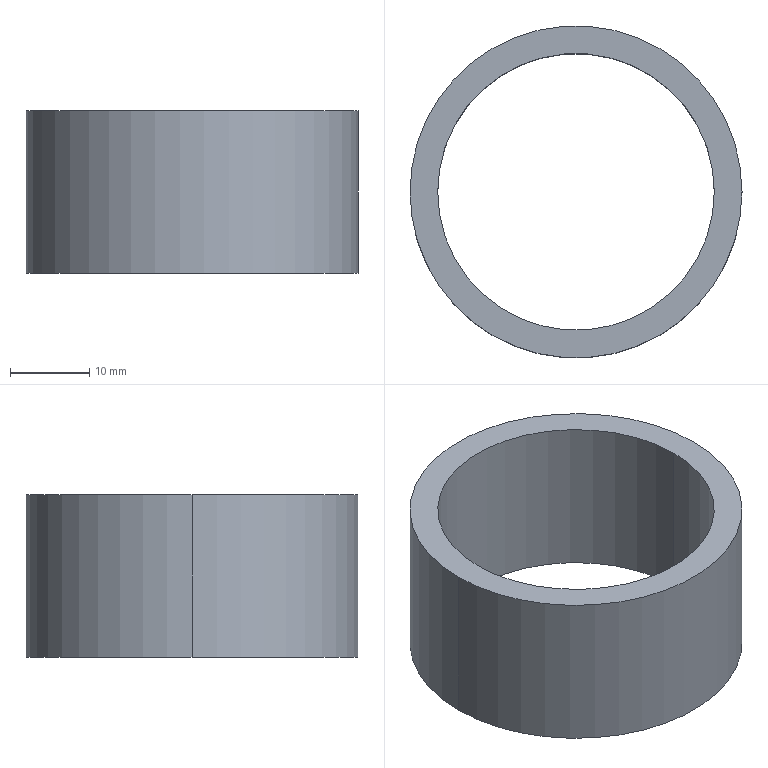Part | STEP file | 01-Spacer 51 | 1 solid | 6 faces | box 42 x 42 x 20.6 mm | volume 8721 mm3 | cylinder 4 | plane 2 | commonest cylinder face diameters 35 x2 42 x2
STEP:
#1=CARTESIAN_POINT('',(0.,0.,0.));
#2=DIRECTION('',(0.,0.,1.));
#3=DIRECTION('',(1.,0.,0.));
#4=AXIS2_PLACEMENT_3D('',#1,#2,#3);
#5=CARTESIAN_POINT('',(-17.5,0.,20.6));
#6=VERTEX_POINT('',#5);
#7=CARTESIAN_POINT('',(-17.5,0.,0.));
#8=VERTEX_POINT('',#7);
#9=CARTESIAN_POINT('',(-17.5,0.,20.6));
#10=DIRECTION('',(0.,0.,-1.));
#11=VECTOR('',#10,1.);
#12=LINE('',#9,#11);
#13=CARTESIAN_POINT('',(0.,0.,20.6));
#14=DIRECTION('',(0.,0.,-1.));
#15=DIRECTION('',(-1.,0.,0.));
#16=AXIS2_PLACEMENT_3D('',#13,#14,#15);
#17=CYLINDRICAL_SURFACE('',#16,17.5);
#18=CARTESIAN_POINT('',(6.283,0.));
#19=DIRECTION('',(0.,1.));
#20=VECTOR('',#19,1.);
#21=LINE('',#18,#20);
#22=(GEOMETRIC_REPRESENTATION_CONTEXT(2)PARAMETRIC_REPRESENTATION_CONTEXT()REPRESENTATION_CONTEXT('',''));
#23=DEFINITIONAL_REPRESENTATION('',(#21),#22);
#24=PCURVE('',#17,#23);
#25=CARTESIAN_POINT('',(0.,0.,20.6));
#26=DIRECTION('',(0.,0.,-1.));
#27=DIRECTION('',(-1.,0.,0.));
#28=AXIS2_PLACEMENT_3D('',#25,#26,#27);
#29=CYLINDRICAL_SURFACE('',#28,17.5);
#30=CARTESIAN_POINT('',(0.,0.));
#31=DIRECTION('',(0.,1.));
#32=VECTOR('',#31,1.);
#33=LINE('',#30,#32);
#34=(GEOMETRIC_REPRESENTATION_CONTEXT(2)PARAMETRIC_REPRESENTATION_CONTEXT()REPRESENTATION_CONTEXT('',''));
#35=DEFINITIONAL_REPRESENTATION('',(#33),#34);
#36=PCURVE('',#29,#35);
#37=SURFACE_CURVE('',#12,(#24,#36),.PCURVE_S1.);
#38=EDGE_CURVE('',#6,#8,#37,.T.);
#39=ORIENTED_EDGE('',*,*,#38,.T.);
#40=CARTESIAN_POINT('',(17.5,0.,0.));
#41=VERTEX_POINT('',#40);
#42=CARTESIAN_POINT('',(0.,0.,0.));
#43=DIRECTION('',(0.,0.,1.));
#44=DIRECTION('',(1.,0.,0.));
#45=AXIS2_PLACEMENT_3D('',#42,#43,#44);
#46=CIRCLE('',#45,17.5);
#47=CARTESIAN_POINT('',(9.425,20.6));
#48=DIRECTION('',(-1.,0.));
#49=VECTOR('',#48,1.);
#50=LINE('',#47,#49);
#51=(GEOMETRIC_REPRESENTATION_CONTEXT(2)PARAMETRIC_REPRESENTATION_CONTEXT()REPRESENTATION_CONTEXT('',''));
#52=DEFINITIONAL_REPRESENTATION('',(#50),#51);
#53=PCURVE('',#17,#52);
#54=CARTESIAN_POINT('',(0.,0.,0.));
#55=DIRECTION('',(0.,0.,1.));
#56=DIRECTION('',(1.,0.,0.));
#57=AXIS2_PLACEMENT_3D('',#54,#55,#56);
#58=PLANE('',#57);
#59=CARTESIAN_POINT('',(0.,0.));
#60=DIRECTION('',(1.,0.));
#61=AXIS2_PLACEMENT_2D('',#59,#60);
#62=CIRCLE('',#61,17.5);
#63=(GEOMETRIC_REPRESENTATION_CONTEXT(2)PARAMETRIC_REPRESENTATION_CONTEXT()REPRESENTATION_CONTEXT('',''));
#64=DEFINITIONAL_REPRESENTATION('',(#62),#63);
#65=PCURVE('',#58,#64);
#66=SURFACE_CURVE('',#46,(#53,#65),.PCURVE_S1.);
#67=EDGE_CURVE('',#8,#41,#66,.T.);
#68=ORIENTED_EDGE('',*,*,#67,.T.);
#69=CARTESIAN_POINT('',(17.5,0.,20.6));
#70=VERTEX_POINT('',#69);
#71=CARTESIAN_POINT('',(17.5,0.,20.6));
#72=DIRECTION('',(0.,0.,-1.));
#73=VECTOR('',#72,1.);
#74=LINE('',#71,#73);
#75=CARTESIAN_POINT('',(3.142,0.));
#76=DIRECTION('',(0.,1.));
#77=VECTOR('',#76,1.);
#78=LINE('',#75,#77);
#79=(GEOMETRIC_REPRESENTATION_CONTEXT(2)PARAMETRIC_REPRESENTATION_CONTEXT()REPRESENTATION_CONTEXT('',''));
#80=DEFINITIONAL_REPRESENTATION('',(#78),#79);
#81=PCURVE('',#17,#80);
#82=CARTESIAN_POINT('',(3.142,0.));
#83=DIRECTION('',(0.,1.));
#84=VECTOR('',#83,1.);
#85=LINE('',#82,#84);
#86=(GEOMETRIC_REPRESENTATION_CONTEXT(2)PARAMETRIC_REPRESENTATION_CONTEXT()REPRESENTATION_CONTEXT('',''));
#87=DEFINITIONAL_REPRESENTATION('',(#85),#86);
#88=PCURVE('',#29,#87);
#89=SURFACE_CURVE('',#74,(#81,#88),.PCURVE_S1.);
#90=EDGE_CURVE('',#70,#41,#89,.T.);
#91=ORIENTED_EDGE('',*,*,#90,.F.);
#92=CARTESIAN_POINT('',(0.,0.,20.6));
#93=DIRECTION('',(0.,0.,1.));
#94=DIRECTION('',(1.,0.,0.));
#95=AXIS2_PLACEMENT_3D('',#92,#93,#94);
#96=CIRCLE('',#95,17.5);
#97=CARTESIAN_POINT('',(9.425,0.));
#98=DIRECTION('',(-1.,0.));
#99=VECTOR('',#98,1.);
#100=LINE('',#97,#99);
#101=(GEOMETRIC_REPRESENTATION_CONTEXT(2)PARAMETRIC_REPRESENTATION_CONTEXT()REPRESENTATION_CONTEXT('',''));
#102=DEFINITIONAL_REPRESENTATION('',(#100),#101);
#103=PCURVE('',#17,#102);
#104=CARTESIAN_POINT('',(0.,0.,20.6));
#105=DIRECTION('',(0.,0.,1.));
#106=DIRECTION('',(1.,0.,0.));
#107=AXIS2_PLACEMENT_3D('',#104,#105,#106);
#108=PLANE('',#107);
#109=CARTESIAN_POINT('',(0.,0.));
#110=DIRECTION('',(1.,0.));
#111=AXIS2_PLACEMENT_2D('',#109,#110);
#112=CIRCLE('',#111,17.5);
#113=(GEOMETRIC_REPRESENTATION_CONTEXT(2)PARAMETRIC_REPRESENTATION_CONTEXT()REPRESENTATION_CONTEXT('',''));
#114=DEFINITIONAL_REPRESENTATION('',(#112),#113);
#115=PCURVE('',#108,#114);
#116=SURFACE_CURVE('',#96,(#103,#115),.PCURVE_S1.);
#117=EDGE_CURVE('',#6,#70,#116,.T.);
#118=ORIENTED_EDGE('',*,*,#117,.F.);
#119=EDGE_LOOP('',(#39,#68,#91,#118));
#120=FACE_BOUND('',#119,.F.);
#121=ADVANCED_FACE('',(#120),#17,.F.);
#122=CARTESIAN_POINT('',(21.,0.,20.6));
#123=VERTEX_POINT('',#122);
#124=CARTESIAN_POINT('',(-21.,0.,20.6));
#125=VERTEX_POINT('',#124);
#126=CARTESIAN_POINT('',(0.,0.,20.6));
#127=DIRECTION('',(0.,0.,1.));
#128=DIRECTION('',(1.,0.,0.));
#129=AXIS2_PLACEMENT_3D('',#126,#127,#128);
#130=CIRCLE('',#129,21.);
#131=CARTESIAN_POINT('',(0.,0.,20.6));
#132=DIRECTION('',(0.,0.,-1.));
#133=DIRECTION('',(-1.,0.,0.));
#134=AXIS2_PLACEMENT_3D('',#131,#132,#133);
#135=CYLINDRICAL_SURFACE('',#134,21.);
#136=CARTESIAN_POINT('',(3.142,0.));
#137=DIRECTION('',(-1.,0.));
#138=VECTOR('',#137,1.);
#139=LINE('',#136,#138);
#140=(GEOMETRIC_REPRESENTATION_CONTEXT(2)PARAMETRIC_REPRESENTATION_CONTEXT()REPRESENTATION_CONTEXT('',''));
#141=DEFINITIONAL_REPRESENTATION('',(#139),#140);
#142=PCURVE('',#135,#141);
#143=CARTESIAN_POINT('',(0.,0.));
#144=DIRECTION('',(1.,0.));
#145=AXIS2_PLACEMENT_2D('',#143,#144);
#146=CIRCLE('',#145,21.);
#147=(GEOMETRIC_REPRESENTATION_CONTEXT(2)PARAMETRIC_REPRESENTATION_CONTEXT()REPRESENTATION_CONTEXT('',''));
#148=DEFINITIONAL_REPRESENTATION('',(#146),#147);
#149=PCURVE('',#108,#148);
#150=SURFACE_CURVE('',#130,(#142,#149),.PCURVE_S1.);
#151=EDGE_CURVE('',#123,#125,#150,.T.);
#152=ORIENTED_EDGE('',*,*,#151,.F.);
#153=CARTESIAN_POINT('',(21.,0.,0.));
#154=VERTEX_POINT('',#153);
#155=CARTESIAN_POINT('',(21.,0.,20.6));
#156=DIRECTION('',(0.,0.,-1.));
#157=VECTOR('',#156,1.);
#158=LINE('',#155,#157);
#159=CARTESIAN_POINT('',(3.142,0.));
#160=DIRECTION('',(0.,1.));
#161=VECTOR('',#160,1.);
#162=LINE('',#159,#161);
#163=(GEOMETRIC_REPRESENTATION_CONTEXT(2)PARAMETRIC_REPRESENTATION_CONTEXT()REPRESENTATION_CONTEXT('',''));
#164=DEFINITIONAL_REPRESENTATION('',(#162),#163);
#165=PCURVE('',#135,#164);
#166=CARTESIAN_POINT('',(0.,0.,20.6));
#167=DIRECTION('',(0.,0.,-1.));
#168=DIRECTION('',(-1.,0.,0.));
#169=AXIS2_PLACEMENT_3D('',#166,#167,#168);
#170=CYLINDRICAL_SURFACE('',#169,21.);
#171=CARTESIAN_POINT('',(3.142,0.));
#172=DIRECTION('',(0.,1.));
#173=VECTOR('',#172,1.);
#174=LINE('',#171,#173);
#175=(GEOMETRIC_REPRESENTATION_CONTEXT(2)PARAMETRIC_REPRESENTATION_CONTEXT()REPRESENTATION_CONTEXT('',''));
#176=DEFINITIONAL_REPRESENTATION('',(#174),#175);
#177=PCURVE('',#170,#176);
#178=SURFACE_CURVE('',#158,(#165,#177),.PCURVE_S1.);
#179=EDGE_CURVE('',#123,#154,#178,.T.);
#180=ORIENTED_EDGE('',*,*,#179,.T.);
#181=CARTESIAN_POINT('',(-21.,0.,0.));
#182=VERTEX_POINT('',#181);
#183=CARTESIAN_POINT('',(0.,0.,0.));
#184=DIRECTION('',(0.,0.,1.));
#185=DIRECTION('',(1.,0.,0.));
#186=AXIS2_PLACEMENT_3D('',#183,#184,#185);
#187=CIRCLE('',#186,21.);
#188=CARTESIAN_POINT('',(3.142,20.6));
#189=DIRECTION('',(-1.,0.));
#190=VECTOR('',#189,1.);
#191=LINE('',#188,#190);
#192=(GEOMETRIC_REPRESENTATION_CONTEXT(2)PARAMETRIC_REPRESENTATION_CONTEXT()REPRESENTATION_CONTEXT('',''));
#193=DEFINITIONAL_REPRESENTATION('',(#191),#192);
#194=PCURVE('',#135,#193);
#195=CARTESIAN_POINT('',(0.,0.));
#196=DIRECTION('',(1.,0.));
#197=AXIS2_PLACEMENT_2D('',#195,#196);
#198=CIRCLE('',#197,21.);
#199=(GEOMETRIC_REPRESENTATION_CONTEXT(2)PARAMETRIC_REPRESENTATION_CONTEXT()REPRESENTATION_CONTEXT('',''));
#200=DEFINITIONAL_REPRESENTATION('',(#198),#199);
#201=PCURVE('',#58,#200);
#202=SURFACE_CURVE('',#187,(#194,#201),.PCURVE_S1.);
#203=EDGE_CURVE('',#154,#182,#202,.T.);
#204=ORIENTED_EDGE('',*,*,#203,.T.);
#205=CARTESIAN_POINT('',(-21.,0.,20.6));
#206=DIRECTION('',(0.,0.,-1.));
#207=VECTOR('',#206,1.);
#208=LINE('',#205,#207);
#209=CARTESIAN_POINT('',(0.,0.));
#210=DIRECTION('',(0.,1.));
#211=VECTOR('',#210,1.);
#212=LINE('',#209,#211);
#213=(GEOMETRIC_REPRESENTATION_CONTEXT(2)PARAMETRIC_REPRESENTATION_CONTEXT()REPRESENTATION_CONTEXT('',''));
#214=DEFINITIONAL_REPRESENTATION('',(#212),#213);
#215=PCURVE('',#135,#214);
#216=CARTESIAN_POINT('',(6.283,0.));
#217=DIRECTION('',(0.,1.));
#218=VECTOR('',#217,1.);
#219=LINE('',#216,#218);
#220=(GEOMETRIC_REPRESENTATION_CONTEXT(2)PARAMETRIC_REPRESENTATION_CONTEXT()REPRESENTATION_CONTEXT('',''));
#221=DEFINITIONAL_REPRESENTATION('',(#219),#220);
#222=PCURVE('',#170,#221);
#223=SURFACE_CURVE('',#208,(#215,#222),.PCURVE_S1.);
#224=EDGE_CURVE('',#125,#182,#223,.T.);
#225=ORIENTED_EDGE('',*,*,#224,.F.);
#226=EDGE_LOOP('',(#152,#180,#204,#225));
#227=FACE_BOUND('',#226,.T.);
#228=ADVANCED_FACE('',(#227),#135,.T.);
#229=CARTESIAN_POINT('',(0.,0.,20.6));
#230=DIRECTION('',(0.,0.,1.));
#231=DIRECTION('',(1.,0.,0.));
#232=AXIS2_PLACEMENT_3D('',#229,#230,#231);
#233=CIRCLE('',#232,21.);
#234=CARTESIAN_POINT('',(0.,0.));
#235=DIRECTION('',(1.,0.));
#236=AXIS2_PLACEMENT_2D('',#234,#235);
#237=CIRCLE('',#236,21.);
#238=(GEOMETRIC_REPRESENTATION_CONTEXT(2)PARAMETRIC_REPRESENTATION_CONTEXT()REPRESENTATION_CONTEXT('',''));
#239=DEFINITIONAL_REPRESENTATION('',(#237),#238);
#240=PCURVE('',#108,#239);
#241=CARTESIAN_POINT('',(9.425,0.));
#242=DIRECTION('',(-1.,0.));
#243=VECTOR('',#242,1.);
#244=LINE('',#241,#243);
#245=(GEOMETRIC_REPRESENTATION_CONTEXT(2)PARAMETRIC_REPRESENTATION_CONTEXT()REPRESENTATION_CONTEXT('',''));
#246=DEFINITIONAL_REPRESENTATION('',(#244),#245);
#247=PCURVE('',#170,#246);
#248=SURFACE_CURVE('',#233,(#240,#247),.PCURVE_S1.);
#249=EDGE_CURVE('',#125,#123,#248,.T.);
#250=ORIENTED_EDGE('',*,*,#249,.T.);
#251=ORIENTED_EDGE('',*,*,#151,.T.);
#252=EDGE_LOOP('',(#250,#251));
#253=FACE_BOUND('',#252,.T.);
#254=ORIENTED_EDGE('',*,*,#117,.F.);
#255=CARTESIAN_POINT('',(0.,0.,20.6));
#256=DIRECTION('',(0.,0.,1.));
#257=DIRECTION('',(1.,0.,0.));
#258=AXIS2_PLACEMENT_3D('',#255,#256,#257);
#259=CIRCLE('',#258,17.5);
#260=CARTESIAN_POINT('',(0.,0.));
#261=DIRECTION('',(1.,0.));
#262=AXIS2_PLACEMENT_2D('',#260,#261);
#263=CIRCLE('',#262,17.5);
#264=(GEOMETRIC_REPRESENTATION_CONTEXT(2)PARAMETRIC_REPRESENTATION_CONTEXT()REPRESENTATION_CONTEXT('',''));
#265=DEFINITIONAL_REPRESENTATION('',(#263),#264);
#266=PCURVE('',#108,#265);
#267=CARTESIAN_POINT('',(3.142,0.));
#268=DIRECTION('',(-1.,0.));
#269=VECTOR('',#268,1.);
#270=LINE('',#267,#269);
#271=(GEOMETRIC_REPRESENTATION_CONTEXT(2)PARAMETRIC_REPRESENTATION_CONTEXT()REPRESENTATION_CONTEXT('',''));
#272=DEFINITIONAL_REPRESENTATION('',(#270),#271);
#273=PCURVE('',#29,#272);
#274=SURFACE_CURVE('',#259,(#266,#273),.PCURVE_S1.);
#275=EDGE_CURVE('',#70,#6,#274,.T.);
#276=ORIENTED_EDGE('',*,*,#275,.F.);
#277=EDGE_LOOP('',(#254,#276));
#278=FACE_BOUND('',#277,.T.);
#279=ADVANCED_FACE('',(#253,#278),#108,.T.);
#280=CARTESIAN_POINT('',(0.,0.,0.));
#281=DIRECTION('',(0.,0.,1.));
#282=DIRECTION('',(1.,0.,0.));
#283=AXIS2_PLACEMENT_3D('',#280,#281,#282);
#284=CIRCLE('',#283,21.);
#285=CARTESIAN_POINT('',(0.,0.));
#286=DIRECTION('',(1.,0.));
#287=AXIS2_PLACEMENT_2D('',#285,#286);
#288=CIRCLE('',#287,21.);
#289=(GEOMETRIC_REPRESENTATION_CONTEXT(2)PARAMETRIC_REPRESENTATION_CONTEXT()REPRESENTATION_CONTEXT('',''));
#290=DEFINITIONAL_REPRESENTATION('',(#288),#289);
#291=PCURVE('',#58,#290);
#292=CARTESIAN_POINT('',(9.425,20.6));
#293=DIRECTION('',(-1.,0.));
#294=VECTOR('',#293,1.);
#295=LINE('',#292,#294);
#296=(GEOMETRIC_REPRESENTATION_CONTEXT(2)PARAMETRIC_REPRESENTATION_CONTEXT()REPRESENTATION_CONTEXT('',''));
#297=DEFINITIONAL_REPRESENTATION('',(#295),#296);
#298=PCURVE('',#170,#297);
#299=SURFACE_CURVE('',#284,(#291,#298),.PCURVE_S1.);
#300=EDGE_CURVE('',#182,#154,#299,.T.);
#301=ORIENTED_EDGE('',*,*,#300,.F.);
#302=ORIENTED_EDGE('',*,*,#203,.F.);
#303=EDGE_LOOP('',(#301,#302));
#304=FACE_BOUND('',#303,.T.);
#305=ORIENTED_EDGE('',*,*,#67,.T.);
#306=CARTESIAN_POINT('',(0.,0.,0.));
#307=DIRECTION('',(0.,0.,1.));
#308=DIRECTION('',(1.,0.,0.));
#309=AXIS2_PLACEMENT_3D('',#306,#307,#308);
#310=CIRCLE('',#309,17.5);
#311=CARTESIAN_POINT('',(0.,0.));
#312=DIRECTION('',(1.,0.));
#313=AXIS2_PLACEMENT_2D('',#311,#312);
#314=CIRCLE('',#313,17.5);
#315=(GEOMETRIC_REPRESENTATION_CONTEXT(2)PARAMETRIC_REPRESENTATION_CONTEXT()REPRESENTATION_CONTEXT('',''));
#316=DEFINITIONAL_REPRESENTATION('',(#314),#315);
#317=PCURVE('',#58,#316);
#318=CARTESIAN_POINT('',(3.142,20.6));
#319=DIRECTION('',(-1.,0.));
#320=VECTOR('',#319,1.);
#321=LINE('',#318,#320);
#322=(GEOMETRIC_REPRESENTATION_CONTEXT(2)PARAMETRIC_REPRESENTATION_CONTEXT()REPRESENTATION_CONTEXT('',''));
#323=DEFINITIONAL_REPRESENTATION('',(#321),#322);
#324=PCURVE('',#29,#323);
#325=SURFACE_CURVE('',#310,(#317,#324),.PCURVE_S1.);
#326=EDGE_CURVE('',#41,#8,#325,.T.);
#327=ORIENTED_EDGE('',*,*,#326,.T.);
#328=EDGE_LOOP('',(#305,#327));
#329=FACE_BOUND('',#328,.T.);
#330=ADVANCED_FACE('',(#304,#329),#58,.F.);
#331=ORIENTED_EDGE('',*,*,#179,.F.);
#332=ORIENTED_EDGE('',*,*,#249,.F.);
#333=ORIENTED_EDGE('',*,*,#224,.T.);
#334=ORIENTED_EDGE('',*,*,#300,.T.);
#335=EDGE_LOOP('',(#331,#332,#333,#334));
#336=FACE_BOUND('',#335,.T.);
#337=ADVANCED_FACE('',(#336),#170,.T.);
#338=ORIENTED_EDGE('',*,*,#326,.T.);
#339=ORIENTED_EDGE('',*,*,#38,.F.);
#340=ORIENTED_EDGE('',*,*,#275,.F.);
#341=ORIENTED_EDGE('',*,*,#90,.T.);
#342=EDGE_LOOP('',(#338,#339,#340,#341));
#343=FACE_BOUND('',#342,.F.);
#344=ADVANCED_FACE('',(#343),#29,.F.);
#345=CLOSED_SHELL('',(#121,#228,#279,#330,#337,#344));
#346=MANIFOLD_SOLID_BREP('',#345);
#347=(LENGTH_UNIT()NAMED_UNIT(*)SI_UNIT(.MILLI.,.METRE.));
#348=UNCERTAINTY_MEASURE_WITH_UNIT(LENGTH_MEASURE(0.0000001),#347,'','');
#349=(NAMED_UNIT(*)PLANE_ANGLE_UNIT()SI_UNIT($,.RADIAN.));
#350=(NAMED_UNIT(*)SI_UNIT($,.STERADIAN.)SOLID_ANGLE_UNIT());
#351=(GEOMETRIC_REPRESENTATION_CONTEXT(3)GLOBAL_UNCERTAINTY_ASSIGNED_CONTEXT((#348))GLOBAL_UNIT_ASSIGNED_CONTEXT((#347,#349,#350))REPRESENTATION_CONTEXT('',''));
#352=ADVANCED_BREP_SHAPE_REPRESENTATION('',(#4,#346),#351);